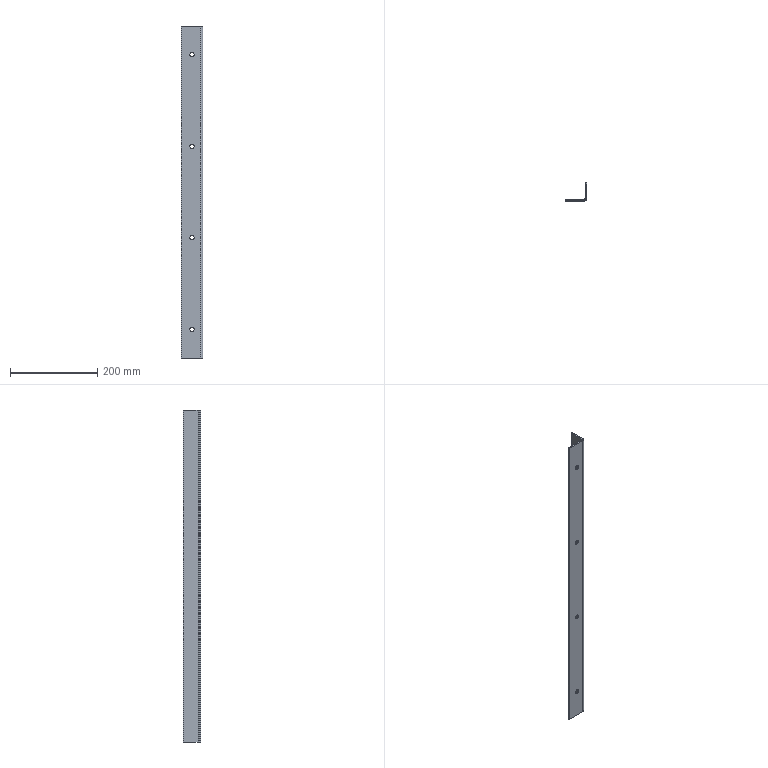Part | STEP file | 750078457 | 1 solid | 18 faces | box 50 x 40 x 762 mm | volume 193524 mm3 | cylinder 10 | plane 8 | commonest cylinder face diameters 10 x8 6 x1 12 x1
STEP:
#1=CARTESIAN_POINT('',(-20.,3.,105.));
#2=VERTEX_POINT('',#1);
#3=CARTESIAN_POINT('',(-30.,3.,105.));
#4=VERTEX_POINT('',#3);
#5=CARTESIAN_POINT('',(-25.,3.,105.));
#6=DIRECTION('',(0.,1.,0.));
#7=DIRECTION('',(1.,0.,0.));
#8=AXIS2_PLACEMENT_3D('',#5,#6,#7);
#9=CIRCLE('',#8,5.);
#10=EDGE_CURVE('',#2,#4,#9,.T.);
#11=ORIENTED_EDGE('',*,*,#10,.T.);
#12=CARTESIAN_POINT('',(-30.,0.,105.));
#13=VERTEX_POINT('',#12);
#14=CARTESIAN_POINT('',(-30.,764.686,105.));
#15=DIRECTION('',(0.,-1.,0.));
#16=VECTOR('',#15,1000.);
#17=LINE('',#14,#16);
#18=EDGE_CURVE('',#4,#13,#17,.T.);
#19=ORIENTED_EDGE('',*,*,#18,.T.);
#20=CARTESIAN_POINT('',(-20.,0.,105.));
#21=VERTEX_POINT('',#20);
#22=CARTESIAN_POINT('',(-25.,0.,105.));
#23=DIRECTION('',(0.,1.,0.));
#24=DIRECTION('',(1.,0.,0.));
#25=AXIS2_PLACEMENT_3D('',#22,#23,#24);
#26=CIRCLE('',#25,5.);
#27=EDGE_CURVE('',#21,#13,#26,.T.);
#28=ORIENTED_EDGE('',*,*,#27,.F.);
#29=CARTESIAN_POINT('',(-20.,764.686,105.));
#30=DIRECTION('',(0.,-1.,0.));
#31=VECTOR('',#30,1000.);
#32=LINE('',#29,#31);
#33=EDGE_CURVE('',#2,#21,#32,.T.);
#34=ORIENTED_EDGE('',*,*,#33,.F.);
#35=EDGE_LOOP('',(#11,#19,#28,#34));
#36=FACE_OUTER_BOUND('',#35,.T.);
#37=CARTESIAN_POINT('',(-25.,764.686,105.));
#38=DIRECTION('',(0.,-1.,0.));
#39=DIRECTION('',(1.,0.,0.));
#40=AXIS2_PLACEMENT_3D('',#37,#38,#39);
#41=CYLINDRICAL_SURFACE('',#40,5.);
#42=ADVANCED_FACE('',(#36),#41,.F.);
#43=CARTESIAN_POINT('',(-20.,3.,-315.));
#44=VERTEX_POINT('',#43);
#45=CARTESIAN_POINT('',(-30.,3.,-315.));
#46=VERTEX_POINT('',#45);
#47=CARTESIAN_POINT('',(-25.,3.,-315.));
#48=DIRECTION('',(0.,1.,0.));
#49=DIRECTION('',(1.,0.,0.));
#50=AXIS2_PLACEMENT_3D('',#47,#48,#49);
#51=CIRCLE('',#50,5.);
#52=EDGE_CURVE('',#44,#46,#51,.T.);
#53=ORIENTED_EDGE('',*,*,#52,.T.);
#54=CARTESIAN_POINT('',(-30.,0.,-315.));
#55=VERTEX_POINT('',#54);
#56=CARTESIAN_POINT('',(-30.,764.686,-315.));
#57=DIRECTION('',(0.,-1.,0.));
#58=VECTOR('',#57,1000.);
#59=LINE('',#56,#58);
#60=EDGE_CURVE('',#46,#55,#59,.T.);
#61=ORIENTED_EDGE('',*,*,#60,.T.);
#62=CARTESIAN_POINT('',(-20.,0.,-315.));
#63=VERTEX_POINT('',#62);
#64=CARTESIAN_POINT('',(-25.,0.,-315.));
#65=DIRECTION('',(0.,1.,0.));
#66=DIRECTION('',(1.,0.,0.));
#67=AXIS2_PLACEMENT_3D('',#64,#65,#66);
#68=CIRCLE('',#67,5.);
#69=EDGE_CURVE('',#63,#55,#68,.T.);
#70=ORIENTED_EDGE('',*,*,#69,.F.);
#71=CARTESIAN_POINT('',(-20.,764.686,-315.));
#72=DIRECTION('',(0.,-1.,0.));
#73=VECTOR('',#72,1000.);
#74=LINE('',#71,#73);
#75=EDGE_CURVE('',#44,#63,#74,.T.);
#76=ORIENTED_EDGE('',*,*,#75,.F.);
#77=EDGE_LOOP('',(#53,#61,#70,#76));
#78=FACE_OUTER_BOUND('',#77,.T.);
#79=CARTESIAN_POINT('',(-25.,764.686,-315.));
#80=DIRECTION('',(0.,-1.,0.));
#81=DIRECTION('',(1.,0.,0.));
#82=AXIS2_PLACEMENT_3D('',#79,#80,#81);
#83=CYLINDRICAL_SURFACE('',#82,5.);
#84=ADVANCED_FACE('',(#78),#83,.F.);
#85=CARTESIAN_POINT('',(-20.,3.,-105.));
#86=VERTEX_POINT('',#85);
#87=CARTESIAN_POINT('',(-30.,3.,-105.));
#88=VERTEX_POINT('',#87);
#89=CARTESIAN_POINT('',(-25.,3.,-105.));
#90=DIRECTION('',(0.,1.,0.));
#91=DIRECTION('',(1.,0.,0.));
#92=AXIS2_PLACEMENT_3D('',#89,#90,#91);
#93=CIRCLE('',#92,5.);
#94=EDGE_CURVE('',#86,#88,#93,.T.);
#95=ORIENTED_EDGE('',*,*,#94,.T.);
#96=CARTESIAN_POINT('',(-30.,0.,-105.));
#97=VERTEX_POINT('',#96);
#98=CARTESIAN_POINT('',(-30.,764.686,-105.));
#99=DIRECTION('',(0.,-1.,0.));
#100=VECTOR('',#99,1000.);
#101=LINE('',#98,#100);
#102=EDGE_CURVE('',#88,#97,#101,.T.);
#103=ORIENTED_EDGE('',*,*,#102,.T.);
#104=CARTESIAN_POINT('',(-20.,0.,-105.));
#105=VERTEX_POINT('',#104);
#106=CARTESIAN_POINT('',(-25.,0.,-105.));
#107=DIRECTION('',(0.,1.,0.));
#108=DIRECTION('',(1.,0.,0.));
#109=AXIS2_PLACEMENT_3D('',#106,#107,#108);
#110=CIRCLE('',#109,5.);
#111=EDGE_CURVE('',#105,#97,#110,.T.);
#112=ORIENTED_EDGE('',*,*,#111,.F.);
#113=CARTESIAN_POINT('',(-20.,764.686,-105.));
#114=DIRECTION('',(0.,-1.,0.));
#115=VECTOR('',#114,1000.);
#116=LINE('',#113,#115);
#117=EDGE_CURVE('',#86,#105,#116,.T.);
#118=ORIENTED_EDGE('',*,*,#117,.F.);
#119=EDGE_LOOP('',(#95,#103,#112,#118));
#120=FACE_OUTER_BOUND('',#119,.T.);
#121=CARTESIAN_POINT('',(-25.,764.686,-105.));
#122=DIRECTION('',(0.,-1.,0.));
#123=DIRECTION('',(1.,0.,0.));
#124=AXIS2_PLACEMENT_3D('',#121,#122,#123);
#125=CYLINDRICAL_SURFACE('',#124,5.);
#126=ADVANCED_FACE('',(#120),#125,.F.);
#127=CARTESIAN_POINT('',(-20.,3.,315.));
#128=VERTEX_POINT('',#127);
#129=CARTESIAN_POINT('',(-30.,3.,315.));
#130=VERTEX_POINT('',#129);
#131=CARTESIAN_POINT('',(-25.,3.,315.));
#132=DIRECTION('',(0.,1.,0.));
#133=DIRECTION('',(1.,0.,0.));
#134=AXIS2_PLACEMENT_3D('',#131,#132,#133);
#135=CIRCLE('',#134,5.);
#136=EDGE_CURVE('',#128,#130,#135,.T.);
#137=ORIENTED_EDGE('',*,*,#136,.T.);
#138=CARTESIAN_POINT('',(-30.,0.,315.));
#139=VERTEX_POINT('',#138);
#140=CARTESIAN_POINT('',(-30.,764.686,315.));
#141=DIRECTION('',(0.,-1.,0.));
#142=VECTOR('',#141,1000.);
#143=LINE('',#140,#142);
#144=EDGE_CURVE('',#130,#139,#143,.T.);
#145=ORIENTED_EDGE('',*,*,#144,.T.);
#146=CARTESIAN_POINT('',(-20.,0.,315.));
#147=VERTEX_POINT('',#146);
#148=CARTESIAN_POINT('',(-25.,0.,315.));
#149=DIRECTION('',(0.,1.,0.));
#150=DIRECTION('',(1.,0.,0.));
#151=AXIS2_PLACEMENT_3D('',#148,#149,#150);
#152=CIRCLE('',#151,5.);
#153=EDGE_CURVE('',#147,#139,#152,.T.);
#154=ORIENTED_EDGE('',*,*,#153,.F.);
#155=CARTESIAN_POINT('',(-20.,764.686,315.));
#156=DIRECTION('',(0.,-1.,0.));
#157=VECTOR('',#156,1000.);
#158=LINE('',#155,#157);
#159=EDGE_CURVE('',#128,#147,#158,.T.);
#160=ORIENTED_EDGE('',*,*,#159,.F.);
#161=EDGE_LOOP('',(#137,#145,#154,#160));
#162=FACE_OUTER_BOUND('',#161,.T.);
#163=CARTESIAN_POINT('',(-25.,764.686,315.));
#164=DIRECTION('',(0.,-1.,0.));
#165=DIRECTION('',(1.,0.,0.));
#166=AXIS2_PLACEMENT_3D('',#163,#164,#165);
#167=CYLINDRICAL_SURFACE('',#166,5.);
#168=ADVANCED_FACE('',(#162),#167,.F.);
#169=CARTESIAN_POINT('',(-50.,3.,381.));
#170=VERTEX_POINT('',#169);
#171=CARTESIAN_POINT('',(-50.,3.,-381.));
#172=VERTEX_POINT('',#171);
#173=CARTESIAN_POINT('',(-50.,3.,381.));
#174=DIRECTION('',(0.,0.,-1.));
#175=VECTOR('',#174,1000.);
#176=LINE('',#173,#175);
#177=EDGE_CURVE('',#170,#172,#176,.T.);
#178=ORIENTED_EDGE('',*,*,#177,.F.);
#179=CARTESIAN_POINT('',(-6.,3.,381.));
#180=VERTEX_POINT('',#179);
#181=CARTESIAN_POINT('',(0.,3.,381.));
#182=DIRECTION('',(-1.,0.,0.));
#183=VECTOR('',#182,1000.);
#184=LINE('',#181,#183);
#185=EDGE_CURVE('',#180,#170,#184,.T.);
#186=ORIENTED_EDGE('',*,*,#185,.F.);
#187=CARTESIAN_POINT('',(-6.,3.,-381.));
#188=VERTEX_POINT('',#187);
#189=CARTESIAN_POINT('',(-6.,3.,381.));
#190=DIRECTION('',(0.,0.,1.));
#191=VECTOR('',#190,1000.);
#192=LINE('',#189,#191);
#193=EDGE_CURVE('',#188,#180,#192,.T.);
#194=ORIENTED_EDGE('',*,*,#193,.F.);
#195=CARTESIAN_POINT('',(0.,3.,-381.));
#196=DIRECTION('',(1.,0.,0.));
#197=VECTOR('',#196,1000.);
#198=LINE('',#195,#197);
#199=EDGE_CURVE('',#172,#188,#198,.T.);
#200=ORIENTED_EDGE('',*,*,#199,.F.);
#201=EDGE_LOOP('',(#178,#186,#194,#200));
#202=FACE_OUTER_BOUND('',#201,.T.);
#203=ORIENTED_EDGE('',*,*,#10,.F.);
#204=CARTESIAN_POINT('',(-25.,3.,105.));
#205=DIRECTION('',(0.,1.,0.));
#206=DIRECTION('',(1.,0.,0.));
#207=AXIS2_PLACEMENT_3D('',#204,#205,#206);
#208=CIRCLE('',#207,5.);
#209=EDGE_CURVE('',#4,#2,#208,.T.);
#210=ORIENTED_EDGE('',*,*,#209,.F.);
#211=EDGE_LOOP('',(#203,#210));
#212=FACE_BOUND('',#211,.T.);
#213=ORIENTED_EDGE('',*,*,#52,.F.);
#214=CARTESIAN_POINT('',(-25.,3.,-315.));
#215=DIRECTION('',(0.,1.,0.));
#216=DIRECTION('',(1.,0.,0.));
#217=AXIS2_PLACEMENT_3D('',#214,#215,#216);
#218=CIRCLE('',#217,5.);
#219=EDGE_CURVE('',#46,#44,#218,.T.);
#220=ORIENTED_EDGE('',*,*,#219,.F.);
#221=EDGE_LOOP('',(#213,#220));
#222=FACE_BOUND('',#221,.T.);
#223=ORIENTED_EDGE('',*,*,#94,.F.);
#224=CARTESIAN_POINT('',(-25.,3.,-105.));
#225=DIRECTION('',(0.,1.,0.));
#226=DIRECTION('',(1.,0.,0.));
#227=AXIS2_PLACEMENT_3D('',#224,#225,#226);
#228=CIRCLE('',#227,5.);
#229=EDGE_CURVE('',#88,#86,#228,.T.);
#230=ORIENTED_EDGE('',*,*,#229,.F.);
#231=EDGE_LOOP('',(#223,#230));
#232=FACE_BOUND('',#231,.T.);
#233=ORIENTED_EDGE('',*,*,#136,.F.);
#234=CARTESIAN_POINT('',(-25.,3.,315.));
#235=DIRECTION('',(0.,1.,0.));
#236=DIRECTION('',(1.,0.,0.));
#237=AXIS2_PLACEMENT_3D('',#234,#235,#236);
#238=CIRCLE('',#237,5.);
#239=EDGE_CURVE('',#130,#128,#238,.T.);
#240=ORIENTED_EDGE('',*,*,#239,.F.);
#241=EDGE_LOOP('',(#233,#240));
#242=FACE_BOUND('',#241,.T.);
#243=CARTESIAN_POINT('',(0.,3.,381.));
#244=DIRECTION('',(0.,-1.,0.));
#245=DIRECTION('',(1.,0.,0.));
#246=AXIS2_PLACEMENT_3D('',#243,#244,#245);
#247=PLANE('',#246);
#248=ADVANCED_FACE('',(#202,#212,#222,#232,#242),#247,.F.);
#249=CARTESIAN_POINT('',(-6.,0.,-381.));
#250=VERTEX_POINT('',#249);
#251=CARTESIAN_POINT('',(0.,6.,-381.));
#252=VERTEX_POINT('',#251);
#253=CARTESIAN_POINT('',(-6.,6.,-381.));
#254=DIRECTION('',(0.,0.,1.));
#255=DIRECTION('',(-1.,0.,0.));
#256=AXIS2_PLACEMENT_3D('',#253,#254,#255);
#257=CIRCLE('',#256,6.);
#258=EDGE_CURVE('',#250,#252,#257,.T.);
#259=ORIENTED_EDGE('',*,*,#258,.F.);
#260=CARTESIAN_POINT('',(-50.,0.,-381.));
#261=VERTEX_POINT('',#260);
#262=CARTESIAN_POINT('',(0.,0.,-381.));
#263=DIRECTION('',(1.,0.,0.));
#264=VECTOR('',#263,1000.);
#265=LINE('',#262,#264);
#266=EDGE_CURVE('',#261,#250,#265,.T.);
#267=ORIENTED_EDGE('',*,*,#266,.F.);
#268=CARTESIAN_POINT('',(-50.,40.,-381.));
#269=DIRECTION('',(0.,-1.,0.));
#270=VECTOR('',#269,1000.);
#271=LINE('',#268,#270);
#272=EDGE_CURVE('',#172,#261,#271,.T.);
#273=ORIENTED_EDGE('',*,*,#272,.F.);
#274=ORIENTED_EDGE('',*,*,#199,.T.);
#275=CARTESIAN_POINT('',(-3.,6.,-381.));
#276=VERTEX_POINT('',#275);
#277=CARTESIAN_POINT('',(-6.,6.,-381.));
#278=DIRECTION('',(0.,0.,-1.));
#279=DIRECTION('',(-1.,0.,0.));
#280=AXIS2_PLACEMENT_3D('',#277,#278,#279);
#281=CIRCLE('',#280,3.);
#282=EDGE_CURVE('',#276,#188,#281,.T.);
#283=ORIENTED_EDGE('',*,*,#282,.F.);
#284=CARTESIAN_POINT('',(-3.,40.,-381.));
#285=VERTEX_POINT('',#284);
#286=CARTESIAN_POINT('',(-3.,40.,-381.));
#287=DIRECTION('',(0.,-1.,0.));
#288=VECTOR('',#287,1000.);
#289=LINE('',#286,#288);
#290=EDGE_CURVE('',#285,#276,#289,.T.);
#291=ORIENTED_EDGE('',*,*,#290,.F.);
#292=CARTESIAN_POINT('',(0.,40.,-381.));
#293=VERTEX_POINT('',#292);
#294=CARTESIAN_POINT('',(0.,40.,-381.));
#295=DIRECTION('',(-1.,0.,0.));
#296=VECTOR('',#295,1000.);
#297=LINE('',#294,#296);
#298=EDGE_CURVE('',#293,#285,#297,.T.);
#299=ORIENTED_EDGE('',*,*,#298,.F.);
#300=CARTESIAN_POINT('',(0.,40.,-381.));
#301=DIRECTION('',(0.,1.,0.));
#302=VECTOR('',#301,1000.);
#303=LINE('',#300,#302);
#304=EDGE_CURVE('',#252,#293,#303,.T.);
#305=ORIENTED_EDGE('',*,*,#304,.F.);
#306=EDGE_LOOP('',(#259,#267,#273,#274,#283,#291,#299,#305));
#307=FACE_OUTER_BOUND('',#306,.T.);
#308=CARTESIAN_POINT('',(0.,40.,-381.));
#309=DIRECTION('',(0.,0.,1.));
#310=DIRECTION('',(1.,0.,0.));
#311=AXIS2_PLACEMENT_3D('',#308,#309,#310);
#312=PLANE('',#311);
#313=ADVANCED_FACE('',(#307),#312,.F.);
#314=ORIENTED_EDGE('',*,*,#272,.T.);
#315=CARTESIAN_POINT('',(-50.,0.,381.));
#316=VERTEX_POINT('',#315);
#317=CARTESIAN_POINT('',(-50.,0.,381.));
#318=DIRECTION('',(0.,0.,1.));
#319=VECTOR('',#318,1000.);
#320=LINE('',#317,#319);
#321=EDGE_CURVE('',#261,#316,#320,.T.);
#322=ORIENTED_EDGE('',*,*,#321,.T.);
#323=CARTESIAN_POINT('',(-50.,0.,381.));
#324=DIRECTION('',(0.,1.,0.));
#325=VECTOR('',#324,1000.);
#326=LINE('',#323,#325);
#327=EDGE_CURVE('',#316,#170,#326,.T.);
#328=ORIENTED_EDGE('',*,*,#327,.T.);
#329=ORIENTED_EDGE('',*,*,#177,.T.);
#330=EDGE_LOOP('',(#314,#322,#328,#329));
#331=FACE_OUTER_BOUND('',#330,.T.);
#332=CARTESIAN_POINT('',(-50.,0.,381.));
#333=DIRECTION('',(-1.,0.,0.));
#334=DIRECTION('',(0.,-1.,0.));
#335=AXIS2_PLACEMENT_3D('',#332,#333,#334);
#336=PLANE('',#335);
#337=ADVANCED_FACE('',(#331),#336,.T.);
#338=ORIENTED_EDGE('',*,*,#185,.T.);
#339=ORIENTED_EDGE('',*,*,#327,.F.);
#340=CARTESIAN_POINT('',(-6.,0.,381.));
#341=VERTEX_POINT('',#340);
#342=CARTESIAN_POINT('',(0.,0.,381.));
#343=DIRECTION('',(1.,0.,0.));
#344=VECTOR('',#343,1000.);
#345=LINE('',#342,#344);
#346=EDGE_CURVE('',#316,#341,#345,.T.);
#347=ORIENTED_EDGE('',*,*,#346,.T.);
#348=CARTESIAN_POINT('',(0.,6.,381.));
#349=VERTEX_POINT('',#348);
#350=CARTESIAN_POINT('',(-6.,6.,381.));
#351=DIRECTION('',(0.,0.,1.));
#352=DIRECTION('',(-1.,0.,0.));
#353=AXIS2_PLACEMENT_3D('',#350,#351,#352);
#354=CIRCLE('',#353,6.);
#355=EDGE_CURVE('',#341,#349,#354,.T.);
#356=ORIENTED_EDGE('',*,*,#355,.T.);
#357=CARTESIAN_POINT('',(0.,40.,381.));
#358=VERTEX_POINT('',#357);
#359=CARTESIAN_POINT('',(0.,0.,381.));
#360=DIRECTION('',(0.,1.,0.));
#361=VECTOR('',#360,1000.);
#362=LINE('',#359,#361);
#363=EDGE_CURVE('',#349,#358,#362,.T.);
#364=ORIENTED_EDGE('',*,*,#363,.T.);
#365=CARTESIAN_POINT('',(-3.,40.,381.));
#366=VERTEX_POINT('',#365);
#367=CARTESIAN_POINT('',(0.,40.,381.));
#368=DIRECTION('',(-1.,0.,0.));
#369=VECTOR('',#368,1000.);
#370=LINE('',#367,#369);
#371=EDGE_CURVE('',#358,#366,#370,.T.);
#372=ORIENTED_EDGE('',*,*,#371,.T.);
#373=CARTESIAN_POINT('',(-3.,6.,381.));
#374=VERTEX_POINT('',#373);
#375=CARTESIAN_POINT('',(-3.,0.,381.));
#376=DIRECTION('',(0.,-1.,0.));
#377=VECTOR('',#376,1000.);
#378=LINE('',#375,#377);
#379=EDGE_CURVE('',#366,#374,#378,.T.);
#380=ORIENTED_EDGE('',*,*,#379,.T.);
#381=CARTESIAN_POINT('',(-6.,6.,381.));
#382=DIRECTION('',(0.,0.,-1.));
#383=DIRECTION('',(-1.,0.,0.));
#384=AXIS2_PLACEMENT_3D('',#381,#382,#383);
#385=CIRCLE('',#384,3.);
#386=EDGE_CURVE('',#374,#180,#385,.T.);
#387=ORIENTED_EDGE('',*,*,#386,.T.);
#388=EDGE_LOOP('',(#338,#339,#347,#356,#364,#372,#380,#387));
#389=FACE_OUTER_BOUND('',#388,.T.);
#390=CARTESIAN_POINT('',(0.,0.,381.));
#391=DIRECTION('',(0.,0.,1.));
#392=DIRECTION('',(1.,0.,0.));
#393=AXIS2_PLACEMENT_3D('',#390,#391,#392);
#394=PLANE('',#393);
#395=ADVANCED_FACE('',(#389),#394,.T.);
#396=ORIENTED_EDGE('',*,*,#193,.T.);
#397=ORIENTED_EDGE('',*,*,#386,.F.);
#398=CARTESIAN_POINT('',(-3.,6.,381.));
#399=DIRECTION('',(0.,0.,1.));
#400=VECTOR('',#399,1000.);
#401=LINE('',#398,#400);
#402=EDGE_CURVE('',#276,#374,#401,.T.);
#403=ORIENTED_EDGE('',*,*,#402,.F.);
#404=ORIENTED_EDGE('',*,*,#282,.T.);
#405=EDGE_LOOP('',(#396,#397,#403,#404));
#406=FACE_OUTER_BOUND('',#405,.T.);
#407=CARTESIAN_POINT('',(-6.,6.,381.));
#408=DIRECTION('',(0.,0.,-1.));
#409=DIRECTION('',(-1.,0.,0.));
#410=AXIS2_PLACEMENT_3D('',#407,#408,#409);
#411=CYLINDRICAL_SURFACE('',#410,3.);
#412=ADVANCED_FACE('',(#406),#411,.F.);
#413=ORIENTED_EDGE('',*,*,#18,.F.);
#414=ORIENTED_EDGE('',*,*,#209,.T.);
#415=ORIENTED_EDGE('',*,*,#33,.T.);
#416=CARTESIAN_POINT('',(-25.,0.,105.));
#417=DIRECTION('',(0.,1.,0.));
#418=DIRECTION('',(1.,0.,0.));
#419=AXIS2_PLACEMENT_3D('',#416,#417,#418);
#420=CIRCLE('',#419,5.);
#421=EDGE_CURVE('',#13,#21,#420,.T.);
#422=ORIENTED_EDGE('',*,*,#421,.F.);
#423=EDGE_LOOP('',(#413,#414,#415,#422));
#424=FACE_OUTER_BOUND('',#423,.T.);
#425=CARTESIAN_POINT('',(-25.,764.686,105.));
#426=DIRECTION('',(0.,-1.,0.));
#427=DIRECTION('',(1.,0.,0.));
#428=AXIS2_PLACEMENT_3D('',#425,#426,#427);
#429=CYLINDRICAL_SURFACE('',#428,5.);
#430=ADVANCED_FACE('',(#424),#429,.F.);
#431=ORIENTED_EDGE('',*,*,#60,.F.);
#432=ORIENTED_EDGE('',*,*,#219,.T.);
#433=ORIENTED_EDGE('',*,*,#75,.T.);
#434=CARTESIAN_POINT('',(-25.,0.,-315.));
#435=DIRECTION('',(0.,1.,0.));
#436=DIRECTION('',(1.,0.,0.));
#437=AXIS2_PLACEMENT_3D('',#434,#435,#436);
#438=CIRCLE('',#437,5.);
#439=EDGE_CURVE('',#55,#63,#438,.T.);
#440=ORIENTED_EDGE('',*,*,#439,.F.);
#441=EDGE_LOOP('',(#431,#432,#433,#440));
#442=FACE_OUTER_BOUND('',#441,.T.);
#443=CARTESIAN_POINT('',(-25.,764.686,-315.));
#444=DIRECTION('',(0.,-1.,0.));
#445=DIRECTION('',(1.,0.,0.));
#446=AXIS2_PLACEMENT_3D('',#443,#444,#445);
#447=CYLINDRICAL_SURFACE('',#446,5.);
#448=ADVANCED_FACE('',(#442),#447,.F.);
#449=ORIENTED_EDGE('',*,*,#102,.F.);
#450=ORIENTED_EDGE('',*,*,#229,.T.);
#451=ORIENTED_EDGE('',*,*,#117,.T.);
#452=CARTESIAN_POINT('',(-25.,0.,-105.));
#453=DIRECTION('',(0.,1.,0.));
#454=DIRECTION('',(1.,0.,0.));
#455=AXIS2_PLACEMENT_3D('',#452,#453,#454);
#456=CIRCLE('',#455,5.);
#457=EDGE_CURVE('',#97,#105,#456,.T.);
#458=ORIENTED_EDGE('',*,*,#457,.F.);
#459=EDGE_LOOP('',(#449,#450,#451,#458));
#460=FACE_OUTER_BOUND('',#459,.T.);
#461=CARTESIAN_POINT('',(-25.,764.686,-105.));
#462=DIRECTION('',(0.,-1.,0.));
#463=DIRECTION('',(1.,0.,0.));
#464=AXIS2_PLACEMENT_3D('',#461,#462,#463);
#465=CYLINDRICAL_SURFACE('',#464,5.);
#466=ADVANCED_FACE('',(#460),#465,.F.);
#467=ORIENTED_EDGE('',*,*,#144,.F.);
#468=ORIENTED_EDGE('',*,*,#239,.T.);
#469=ORIENTED_EDGE('',*,*,#159,.T.);
#470=CARTESIAN_POINT('',(-25.,0.,315.));
#471=DIRECTION('',(0.,1.,0.));
#472=DIRECTION('',(1.,0.,0.));
#473=AXIS2_PLACEMENT_3D('',#470,#471,#472);
#474=CIRCLE('',#473,5.);
#475=EDGE_CURVE('',#139,#147,#474,.T.);
#476=ORIENTED_EDGE('',*,*,#475,.F.);
#477=EDGE_LOOP('',(#467,#468,#469,#476));
#478=FACE_OUTER_BOUND('',#477,.T.);
#479=CARTESIAN_POINT('',(-25.,764.686,315.));
#480=DIRECTION('',(0.,-1.,0.));
#481=DIRECTION('',(1.,0.,0.));
#482=AXIS2_PLACEMENT_3D('',#479,#480,#481);
#483=CYLINDRICAL_SURFACE('',#482,5.);
#484=ADVANCED_FACE('',(#478),#483,.F.);
#485=ORIENTED_EDGE('',*,*,#363,.F.);
#486=CARTESIAN_POINT('',(0.,6.,381.));
#487=DIRECTION('',(0.,0.,-1.));
#488=VECTOR('',#487,1000.);
#489=LINE('',#486,#488);
#490=EDGE_CURVE('',#349,#252,#489,.T.);
#491=ORIENTED_EDGE('',*,*,#490,.T.);
#492=ORIENTED_EDGE('',*,*,#304,.T.);
#493=CARTESIAN_POINT('',(0.,40.,381.));
#494=DIRECTION('',(0.,0.,1.));
#495=VECTOR('',#494,1000.);
#496=LINE('',#493,#495);
#497=EDGE_CURVE('',#293,#358,#496,.T.);
#498=ORIENTED_EDGE('',*,*,#497,.T.);
#499=EDGE_LOOP('',(#485,#491,#492,#498));
#500=FACE_OUTER_BOUND('',#499,.T.);
#501=CARTESIAN_POINT('',(0.,40.,381.));
#502=DIRECTION('',(1.,0.,0.));
#503=DIRECTION('',(0.,0.,-1.));
#504=AXIS2_PLACEMENT_3D('',#501,#502,#503);
#505=PLANE('',#504);
#506=ADVANCED_FACE('',(#500),#505,.T.);
#507=ORIENTED_EDGE('',*,*,#355,.F.);
#508=CARTESIAN_POINT('',(-6.,0.,381.));
#509=DIRECTION('',(0.,0.,-1.));
#510=VECTOR('',#509,1000.);
#511=LINE('',#508,#510);
#512=EDGE_CURVE('',#341,#250,#511,.T.);
#513=ORIENTED_EDGE('',*,*,#512,.T.);
#514=ORIENTED_EDGE('',*,*,#258,.T.);
#515=ORIENTED_EDGE('',*,*,#490,.F.);
#516=EDGE_LOOP('',(#507,#513,#514,#515));
#517=FACE_OUTER_BOUND('',#516,.T.);
#518=CARTESIAN_POINT('',(-6.,6.,381.));
#519=DIRECTION('',(0.,0.,-1.));
#520=DIRECTION('',(-1.,0.,0.));
#521=AXIS2_PLACEMENT_3D('',#518,#519,#520);
#522=CYLINDRICAL_SURFACE('',#521,6.);
#523=ADVANCED_FACE('',(#517),#522,.T.);
#524=ORIENTED_EDGE('',*,*,#346,.F.);
#525=ORIENTED_EDGE('',*,*,#321,.F.);
#526=ORIENTED_EDGE('',*,*,#266,.T.);
#527=ORIENTED_EDGE('',*,*,#512,.F.);
#528=EDGE_LOOP('',(#524,#525,#526,#527));
#529=FACE_OUTER_BOUND('',#528,.T.);
#530=ORIENTED_EDGE('',*,*,#27,.T.);
#531=ORIENTED_EDGE('',*,*,#421,.T.);
#532=EDGE_LOOP('',(#530,#531));
#533=FACE_BOUND('',#532,.T.);
#534=ORIENTED_EDGE('',*,*,#69,.T.);
#535=ORIENTED_EDGE('',*,*,#439,.T.);
#536=EDGE_LOOP('',(#534,#535));
#537=FACE_BOUND('',#536,.T.);
#538=ORIENTED_EDGE('',*,*,#111,.T.);
#539=ORIENTED_EDGE('',*,*,#457,.T.);
#540=EDGE_LOOP('',(#538,#539));
#541=FACE_BOUND('',#540,.T.);
#542=ORIENTED_EDGE('',*,*,#153,.T.);
#543=ORIENTED_EDGE('',*,*,#475,.T.);
#544=EDGE_LOOP('',(#542,#543));
#545=FACE_BOUND('',#544,.T.);
#546=CARTESIAN_POINT('',(0.,0.,381.));
#547=DIRECTION('',(0.,-1.,0.));
#548=DIRECTION('',(1.,0.,0.));
#549=AXIS2_PLACEMENT_3D('',#546,#547,#548);
#550=PLANE('',#549);
#551=ADVANCED_FACE('',(#529,#533,#537,#541,#545),#550,.T.);
#552=ORIENTED_EDGE('',*,*,#402,.T.);
#553=ORIENTED_EDGE('',*,*,#379,.F.);
#554=CARTESIAN_POINT('',(-3.,40.,381.));
#555=DIRECTION('',(0.,0.,1.));
#556=VECTOR('',#555,1000.);
#557=LINE('',#554,#556);
#558=EDGE_CURVE('',#285,#366,#557,.T.);
#559=ORIENTED_EDGE('',*,*,#558,.F.);
#560=ORIENTED_EDGE('',*,*,#290,.T.);
#561=EDGE_LOOP('',(#552,#553,#559,#560));
#562=FACE_OUTER_BOUND('',#561,.T.);
#563=CARTESIAN_POINT('',(-3.,40.,381.));
#564=DIRECTION('',(1.,0.,0.));
#565=DIRECTION('',(0.,0.,-1.));
#566=AXIS2_PLACEMENT_3D('',#563,#564,#565);
#567=PLANE('',#566);
#568=ADVANCED_FACE('',(#562),#567,.F.);
#569=ORIENTED_EDGE('',*,*,#371,.F.);
#570=ORIENTED_EDGE('',*,*,#497,.F.);
#571=ORIENTED_EDGE('',*,*,#298,.T.);
#572=ORIENTED_EDGE('',*,*,#558,.T.);
#573=EDGE_LOOP('',(#569,#570,#571,#572));
#574=FACE_OUTER_BOUND('',#573,.T.);
#575=CARTESIAN_POINT('',(0.,40.,381.));
#576=DIRECTION('',(0.,-1.,0.));
#577=DIRECTION('',(0.,0.,-1.));
#578=AXIS2_PLACEMENT_3D('',#575,#576,#577);
#579=PLANE('',#578);
#580=ADVANCED_FACE('',(#574),#579,.F.);
#581=CLOSED_SHELL('',(#42,#84,#126,#168,#248,#313,#337,#395,#412,#430,#448,#466,#484,#506,#523,#551,#568,#580));
#582=MANIFOLD_SOLID_BREP('',#581);
#583=CARTESIAN_POINT('',(0.,0.,0.));
#584=DIRECTION('',(0.,0.,1.));
#585=DIRECTION('',(1.,0.,0.));
#586=AXIS2_PLACEMENT_3D('',#583,#584,#585);
#587=(LENGTH_UNIT()NAMED_UNIT(*)SI_UNIT(.MILLI.,.METRE.));
#588=UNCERTAINTY_MEASURE_WITH_UNIT(LENGTH_MEASURE(0.00001),#587,'','');
#589=(NAMED_UNIT(*)PLANE_ANGLE_UNIT()SI_UNIT($,.RADIAN.));
#590=(NAMED_UNIT(*)SI_UNIT($,.STERADIAN.)SOLID_ANGLE_UNIT());
#591=(GEOMETRIC_REPRESENTATION_CONTEXT(3)GLOBAL_UNCERTAINTY_ASSIGNED_CONTEXT((#588))GLOBAL_UNIT_ASSIGNED_CONTEXT((#587,#589,#590))REPRESENTATION_CONTEXT('',''));
#592=ADVANCED_BREP_SHAPE_REPRESENTATION('',(#582,#586),#591);